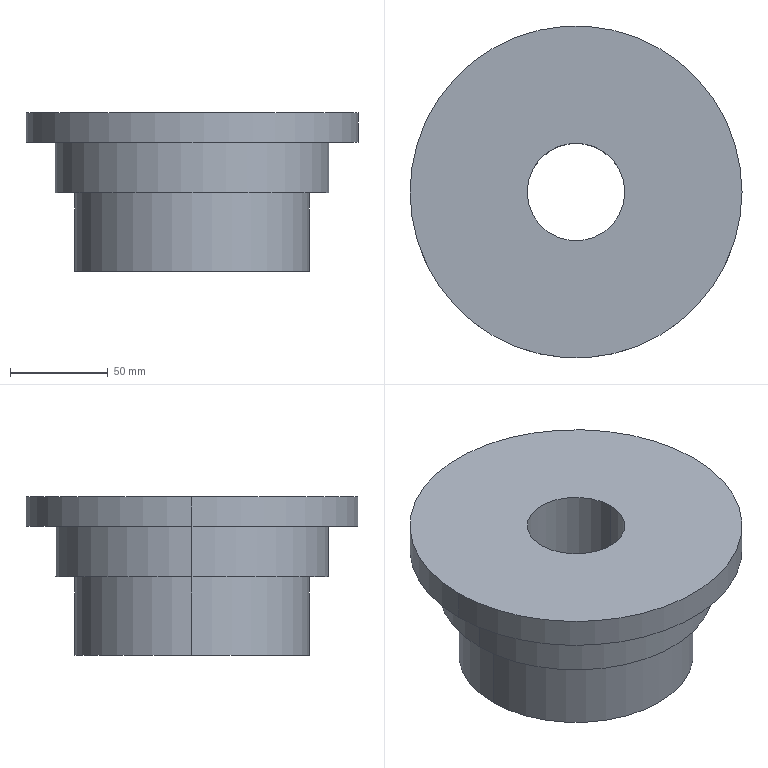Part | SolidWorks | features ICE 2, Cut 1, Extrusion 1 | 1 solid | 12 faces | box 170 x 170 x 81 mm | volume 1034055 mm3 | cylinder 8 | plane 4 | commonest cylinder face diameters 50 x2 120 x2 140 x2 170 x2
STEP:
#1=CARTESIAN_POINT('',(-25.,0.,-40.));
#2=VERTEX_POINT('',#1);
#3=CARTESIAN_POINT('',(25.,0.,-40.));
#4=VERTEX_POINT('',#3);
#5=CARTESIAN_POINT('',(0.,0.,-40.));
#6=DIRECTION('',(0.,0.,1.));
#7=DIRECTION('',(1.,0.,0.));
#8=AXIS2_PLACEMENT_3D('',#5,#6,#7);
#9=CIRCLE('',#8,25.);
#10=EDGE_CURVE('',#2,#4,#9,.T.);
#11=ORIENTED_EDGE('',*,*,#10,.F.);
#12=CARTESIAN_POINT('',(-25.,0.,41.));
#13=VERTEX_POINT('',#12);
#14=CARTESIAN_POINT('',(-25.,0.,-40.));
#15=DIRECTION('',(0.,0.,1.));
#16=VECTOR('',#15,1000.);
#17=LINE('',#14,#16);
#18=EDGE_CURVE('',#2,#13,#17,.T.);
#19=ORIENTED_EDGE('',*,*,#18,.T.);
#20=CARTESIAN_POINT('',(25.,0.,41.));
#21=VERTEX_POINT('',#20);
#22=CARTESIAN_POINT('',(0.,0.,41.));
#23=DIRECTION('',(0.,0.,1.));
#24=DIRECTION('',(1.,0.,0.));
#25=AXIS2_PLACEMENT_3D('',#22,#23,#24);
#26=CIRCLE('',#25,25.);
#27=EDGE_CURVE('',#13,#21,#26,.T.);
#28=ORIENTED_EDGE('',*,*,#27,.T.);
#29=CARTESIAN_POINT('',(25.,0.,-40.));
#30=DIRECTION('',(0.,0.,1.));
#31=VECTOR('',#30,1000.);
#32=LINE('',#29,#31);
#33=EDGE_CURVE('',#4,#21,#32,.T.);
#34=ORIENTED_EDGE('',*,*,#33,.F.);
#35=EDGE_LOOP('',(#11,#19,#28,#34));
#36=FACE_OUTER_BOUND('',#35,.T.);
#37=CARTESIAN_POINT('',(0.,0.,-40.));
#38=DIRECTION('',(0.,0.,1.));
#39=DIRECTION('',(1.,0.,0.));
#40=AXIS2_PLACEMENT_3D('',#37,#38,#39);
#41=CYLINDRICAL_SURFACE('',#40,25.);
#42=ADVANCED_FACE('',(#36),#41,.F.);
#43=CARTESIAN_POINT('',(-60.,0.,-40.));
#44=VERTEX_POINT('',#43);
#45=CARTESIAN_POINT('',(60.,0.,-40.));
#46=VERTEX_POINT('',#45);
#47=CARTESIAN_POINT('',(0.,0.,-40.));
#48=DIRECTION('',(0.,0.,-1.));
#49=DIRECTION('',(-1.,0.,0.));
#50=AXIS2_PLACEMENT_3D('',#47,#48,#49);
#51=CIRCLE('',#50,60.);
#52=EDGE_CURVE('',#44,#46,#51,.T.);
#53=ORIENTED_EDGE('',*,*,#52,.F.);
#54=CARTESIAN_POINT('',(-60.,0.,0.));
#55=VERTEX_POINT('',#54);
#56=CARTESIAN_POINT('',(-60.,0.,-40.));
#57=DIRECTION('',(0.,0.,1.));
#58=VECTOR('',#57,1000.);
#59=LINE('',#56,#58);
#60=EDGE_CURVE('',#44,#55,#59,.T.);
#61=ORIENTED_EDGE('',*,*,#60,.T.);
#62=CARTESIAN_POINT('',(60.,0.,0.));
#63=VERTEX_POINT('',#62);
#64=CARTESIAN_POINT('',(0.,0.,0.));
#65=DIRECTION('',(0.,0.,-1.));
#66=DIRECTION('',(-1.,0.,0.));
#67=AXIS2_PLACEMENT_3D('',#64,#65,#66);
#68=CIRCLE('',#67,60.);
#69=EDGE_CURVE('',#55,#63,#68,.T.);
#70=ORIENTED_EDGE('',*,*,#69,.T.);
#71=CARTESIAN_POINT('',(60.,0.,-40.));
#72=DIRECTION('',(0.,0.,1.));
#73=VECTOR('',#72,1000.);
#74=LINE('',#71,#73);
#75=EDGE_CURVE('',#46,#63,#74,.T.);
#76=ORIENTED_EDGE('',*,*,#75,.F.);
#77=EDGE_LOOP('',(#53,#61,#70,#76));
#78=FACE_OUTER_BOUND('',#77,.T.);
#79=CARTESIAN_POINT('',(0.,0.,-40.));
#80=DIRECTION('',(0.,0.,1.));
#81=DIRECTION('',(1.,0.,0.));
#82=AXIS2_PLACEMENT_3D('',#79,#80,#81);
#83=CYLINDRICAL_SURFACE('',#82,60.);
#84=ADVANCED_FACE('',(#78),#83,.T.);
#85=CARTESIAN_POINT('',(85.,0.,41.));
#86=VERTEX_POINT('',#85);
#87=CARTESIAN_POINT('',(-85.,0.,41.));
#88=VERTEX_POINT('',#87);
#89=CARTESIAN_POINT('',(0.,0.,41.));
#90=DIRECTION('',(0.,0.,1.));
#91=DIRECTION('',(1.,0.,0.));
#92=AXIS2_PLACEMENT_3D('',#89,#90,#91);
#93=CIRCLE('',#92,85.);
#94=EDGE_CURVE('',#86,#88,#93,.T.);
#95=ORIENTED_EDGE('',*,*,#94,.F.);
#96=CARTESIAN_POINT('',(85.,0.,26.));
#97=VERTEX_POINT('',#96);
#98=CARTESIAN_POINT('',(85.,0.,41.));
#99=DIRECTION('',(0.,0.,-1.));
#100=VECTOR('',#99,1000.);
#101=LINE('',#98,#100);
#102=EDGE_CURVE('',#86,#97,#101,.T.);
#103=ORIENTED_EDGE('',*,*,#102,.T.);
#104=CARTESIAN_POINT('',(-85.,0.,26.));
#105=VERTEX_POINT('',#104);
#106=CARTESIAN_POINT('',(0.,0.,26.));
#107=DIRECTION('',(0.,0.,1.));
#108=DIRECTION('',(1.,0.,0.));
#109=AXIS2_PLACEMENT_3D('',#106,#107,#108);
#110=CIRCLE('',#109,85.);
#111=EDGE_CURVE('',#97,#105,#110,.T.);
#112=ORIENTED_EDGE('',*,*,#111,.T.);
#113=CARTESIAN_POINT('',(-85.,0.,41.));
#114=DIRECTION('',(0.,0.,-1.));
#115=VECTOR('',#114,1000.);
#116=LINE('',#113,#115);
#117=EDGE_CURVE('',#88,#105,#116,.T.);
#118=ORIENTED_EDGE('',*,*,#117,.F.);
#119=EDGE_LOOP('',(#95,#103,#112,#118));
#120=FACE_OUTER_BOUND('',#119,.T.);
#121=CARTESIAN_POINT('',(0.,0.,41.));
#122=DIRECTION('',(0.,0.,-1.));
#123=DIRECTION('',(-1.,0.,0.));
#124=AXIS2_PLACEMENT_3D('',#121,#122,#123);
#125=CYLINDRICAL_SURFACE('',#124,85.);
#126=ADVANCED_FACE('',(#120),#125,.T.);
#127=CARTESIAN_POINT('',(70.,0.,26.));
#128=VERTEX_POINT('',#127);
#129=CARTESIAN_POINT('',(-70.,0.,26.));
#130=VERTEX_POINT('',#129);
#131=CARTESIAN_POINT('',(0.,0.,26.));
#132=DIRECTION('',(0.,0.,1.));
#133=DIRECTION('',(1.,0.,0.));
#134=AXIS2_PLACEMENT_3D('',#131,#132,#133);
#135=CIRCLE('',#134,70.);
#136=EDGE_CURVE('',#128,#130,#135,.T.);
#137=ORIENTED_EDGE('',*,*,#136,.F.);
#138=CARTESIAN_POINT('',(70.,0.,0.));
#139=VERTEX_POINT('',#138);
#140=CARTESIAN_POINT('',(70.,0.,223.99));
#141=DIRECTION('',(0.,0.,-1.));
#142=VECTOR('',#141,1000.);
#143=LINE('',#140,#142);
#144=EDGE_CURVE('',#128,#139,#143,.T.);
#145=ORIENTED_EDGE('',*,*,#144,.T.);
#146=CARTESIAN_POINT('',(-70.,0.,0.));
#147=VERTEX_POINT('',#146);
#148=CARTESIAN_POINT('',(0.,0.,0.));
#149=DIRECTION('',(0.,0.,1.));
#150=DIRECTION('',(1.,0.,0.));
#151=AXIS2_PLACEMENT_3D('',#148,#149,#150);
#152=CIRCLE('',#151,70.);
#153=EDGE_CURVE('',#139,#147,#152,.T.);
#154=ORIENTED_EDGE('',*,*,#153,.T.);
#155=CARTESIAN_POINT('',(-70.,0.,223.99));
#156=DIRECTION('',(0.,0.,-1.));
#157=VECTOR('',#156,1000.);
#158=LINE('',#155,#157);
#159=EDGE_CURVE('',#130,#147,#158,.T.);
#160=ORIENTED_EDGE('',*,*,#159,.F.);
#161=EDGE_LOOP('',(#137,#145,#154,#160));
#162=FACE_OUTER_BOUND('',#161,.T.);
#163=CARTESIAN_POINT('',(0.,0.,223.99));
#164=DIRECTION('',(0.,0.,-1.));
#165=DIRECTION('',(-1.,0.,0.));
#166=AXIS2_PLACEMENT_3D('',#163,#164,#165);
#167=CYLINDRICAL_SURFACE('',#166,70.);
#168=ADVANCED_FACE('',(#162),#167,.T.);
#169=ORIENTED_EDGE('',*,*,#144,.F.);
#170=CARTESIAN_POINT('',(0.,0.,26.));
#171=DIRECTION('',(0.,0.,1.));
#172=DIRECTION('',(1.,0.,0.));
#173=AXIS2_PLACEMENT_3D('',#170,#171,#172);
#174=CIRCLE('',#173,70.);
#175=EDGE_CURVE('',#130,#128,#174,.T.);
#176=ORIENTED_EDGE('',*,*,#175,.F.);
#177=ORIENTED_EDGE('',*,*,#159,.T.);
#178=CARTESIAN_POINT('',(0.,0.,0.));
#179=DIRECTION('',(0.,0.,1.));
#180=DIRECTION('',(1.,0.,0.));
#181=AXIS2_PLACEMENT_3D('',#178,#179,#180);
#182=CIRCLE('',#181,70.);
#183=EDGE_CURVE('',#147,#139,#182,.T.);
#184=ORIENTED_EDGE('',*,*,#183,.T.);
#185=EDGE_LOOP('',(#169,#176,#177,#184));
#186=FACE_OUTER_BOUND('',#185,.T.);
#187=CARTESIAN_POINT('',(0.,0.,223.99));
#188=DIRECTION('',(0.,0.,-1.));
#189=DIRECTION('',(-1.,0.,0.));
#190=AXIS2_PLACEMENT_3D('',#187,#188,#189);
#191=CYLINDRICAL_SURFACE('',#190,70.);
#192=ADVANCED_FACE('',(#186),#191,.T.);
#193=CARTESIAN_POINT('',(0.,0.,0.));
#194=DIRECTION('',(0.,0.,-1.));
#195=DIRECTION('',(-1.,0.,0.));
#196=AXIS2_PLACEMENT_3D('',#193,#194,#195);
#197=CIRCLE('',#196,60.);
#198=EDGE_CURVE('',#63,#55,#197,.T.);
#199=ORIENTED_EDGE('',*,*,#198,.F.);
#200=ORIENTED_EDGE('',*,*,#69,.F.);
#201=EDGE_LOOP('',(#199,#200));
#202=FACE_BOUND('',#201,.T.);
#203=ORIENTED_EDGE('',*,*,#183,.F.);
#204=ORIENTED_EDGE('',*,*,#153,.F.);
#205=EDGE_LOOP('',(#203,#204));
#206=FACE_OUTER_BOUND('',#205,.T.);
#207=CARTESIAN_POINT('',(0.,0.,0.));
#208=DIRECTION('',(0.,0.,1.));
#209=DIRECTION('',(1.,0.,0.));
#210=AXIS2_PLACEMENT_3D('',#207,#208,#209);
#211=PLANE('',#210);
#212=ADVANCED_FACE('',(#202,#206),#211,.F.);
#213=ORIENTED_EDGE('',*,*,#102,.F.);
#214=CARTESIAN_POINT('',(0.,0.,41.));
#215=DIRECTION('',(0.,0.,1.));
#216=DIRECTION('',(1.,0.,0.));
#217=AXIS2_PLACEMENT_3D('',#214,#215,#216);
#218=CIRCLE('',#217,85.);
#219=EDGE_CURVE('',#88,#86,#218,.T.);
#220=ORIENTED_EDGE('',*,*,#219,.F.);
#221=ORIENTED_EDGE('',*,*,#117,.T.);
#222=CARTESIAN_POINT('',(0.,0.,26.));
#223=DIRECTION('',(0.,0.,1.));
#224=DIRECTION('',(1.,0.,0.));
#225=AXIS2_PLACEMENT_3D('',#222,#223,#224);
#226=CIRCLE('',#225,85.);
#227=EDGE_CURVE('',#105,#97,#226,.T.);
#228=ORIENTED_EDGE('',*,*,#227,.T.);
#229=EDGE_LOOP('',(#213,#220,#221,#228));
#230=FACE_OUTER_BOUND('',#229,.T.);
#231=CARTESIAN_POINT('',(0.,0.,41.));
#232=DIRECTION('',(0.,0.,-1.));
#233=DIRECTION('',(-1.,0.,0.));
#234=AXIS2_PLACEMENT_3D('',#231,#232,#233);
#235=CYLINDRICAL_SURFACE('',#234,85.);
#236=ADVANCED_FACE('',(#230),#235,.T.);
#237=CARTESIAN_POINT('',(0.,0.,41.));
#238=DIRECTION('',(0.,0.,1.));
#239=DIRECTION('',(1.,0.,0.));
#240=AXIS2_PLACEMENT_3D('',#237,#238,#239);
#241=CIRCLE('',#240,25.);
#242=EDGE_CURVE('',#21,#13,#241,.T.);
#243=ORIENTED_EDGE('',*,*,#242,.F.);
#244=ORIENTED_EDGE('',*,*,#27,.F.);
#245=EDGE_LOOP('',(#243,#244));
#246=FACE_BOUND('',#245,.T.);
#247=ORIENTED_EDGE('',*,*,#219,.T.);
#248=ORIENTED_EDGE('',*,*,#94,.T.);
#249=EDGE_LOOP('',(#247,#248));
#250=FACE_OUTER_BOUND('',#249,.T.);
#251=CARTESIAN_POINT('',(0.,0.,41.));
#252=DIRECTION('',(0.,0.,1.));
#253=DIRECTION('',(1.,0.,0.));
#254=AXIS2_PLACEMENT_3D('',#251,#252,#253);
#255=PLANE('',#254);
#256=ADVANCED_FACE('',(#246,#250),#255,.T.);
#257=ORIENTED_EDGE('',*,*,#175,.T.);
#258=ORIENTED_EDGE('',*,*,#136,.T.);
#259=EDGE_LOOP('',(#257,#258));
#260=FACE_BOUND('',#259,.T.);
#261=ORIENTED_EDGE('',*,*,#227,.F.);
#262=ORIENTED_EDGE('',*,*,#111,.F.);
#263=EDGE_LOOP('',(#261,#262));
#264=FACE_OUTER_BOUND('',#263,.T.);
#265=CARTESIAN_POINT('',(0.,0.,26.));
#266=DIRECTION('',(0.,0.,1.));
#267=DIRECTION('',(1.,0.,0.));
#268=AXIS2_PLACEMENT_3D('',#265,#266,#267);
#269=PLANE('',#268);
#270=ADVANCED_FACE('',(#260,#264),#269,.F.);
#271=ORIENTED_EDGE('',*,*,#60,.F.);
#272=CARTESIAN_POINT('',(0.,0.,-40.));
#273=DIRECTION('',(0.,0.,-1.));
#274=DIRECTION('',(-1.,0.,0.));
#275=AXIS2_PLACEMENT_3D('',#272,#273,#274);
#276=CIRCLE('',#275,60.);
#277=EDGE_CURVE('',#46,#44,#276,.T.);
#278=ORIENTED_EDGE('',*,*,#277,.F.);
#279=ORIENTED_EDGE('',*,*,#75,.T.);
#280=ORIENTED_EDGE('',*,*,#198,.T.);
#281=EDGE_LOOP('',(#271,#278,#279,#280));
#282=FACE_OUTER_BOUND('',#281,.T.);
#283=CARTESIAN_POINT('',(0.,0.,-40.));
#284=DIRECTION('',(0.,0.,1.));
#285=DIRECTION('',(1.,0.,0.));
#286=AXIS2_PLACEMENT_3D('',#283,#284,#285);
#287=CYLINDRICAL_SURFACE('',#286,60.);
#288=ADVANCED_FACE('',(#282),#287,.T.);
#289=CARTESIAN_POINT('',(0.,0.,-40.));
#290=DIRECTION('',(0.,0.,1.));
#291=DIRECTION('',(1.,0.,0.));
#292=AXIS2_PLACEMENT_3D('',#289,#290,#291);
#293=CIRCLE('',#292,25.);
#294=EDGE_CURVE('',#4,#2,#293,.T.);
#295=ORIENTED_EDGE('',*,*,#294,.T.);
#296=ORIENTED_EDGE('',*,*,#10,.T.);
#297=EDGE_LOOP('',(#295,#296));
#298=FACE_BOUND('',#297,.T.);
#299=ORIENTED_EDGE('',*,*,#277,.T.);
#300=ORIENTED_EDGE('',*,*,#52,.T.);
#301=EDGE_LOOP('',(#299,#300));
#302=FACE_OUTER_BOUND('',#301,.T.);
#303=CARTESIAN_POINT('',(0.,0.,-40.));
#304=DIRECTION('',(0.,0.,-1.));
#305=DIRECTION('',(-1.,0.,0.));
#306=AXIS2_PLACEMENT_3D('',#303,#304,#305);
#307=PLANE('',#306);
#308=ADVANCED_FACE('',(#298,#302),#307,.T.);
#309=ORIENTED_EDGE('',*,*,#18,.F.);
#310=ORIENTED_EDGE('',*,*,#294,.F.);
#311=ORIENTED_EDGE('',*,*,#33,.T.);
#312=ORIENTED_EDGE('',*,*,#242,.T.);
#313=EDGE_LOOP('',(#309,#310,#311,#312));
#314=FACE_OUTER_BOUND('',#313,.T.);
#315=CARTESIAN_POINT('',(0.,0.,-40.));
#316=DIRECTION('',(0.,0.,1.));
#317=DIRECTION('',(1.,0.,0.));
#318=AXIS2_PLACEMENT_3D('',#315,#316,#317);
#319=CYLINDRICAL_SURFACE('',#318,25.);
#320=ADVANCED_FACE('',(#314),#319,.F.);
#321=CLOSED_SHELL('',(#42,#84,#126,#168,#192,#212,#236,#256,#270,#288,#308,#320));
#322=MANIFOLD_SOLID_BREP('',#321);
#323=CARTESIAN_POINT('',(0.,0.,0.));
#324=DIRECTION('',(0.,0.,1.));
#325=DIRECTION('',(1.,0.,0.));
#326=AXIS2_PLACEMENT_3D('',#323,#324,#325);
#327=(LENGTH_UNIT()NAMED_UNIT(*)SI_UNIT(.MILLI.,.METRE.));
#328=UNCERTAINTY_MEASURE_WITH_UNIT(LENGTH_MEASURE(0.00001),#327,'','');
#329=(NAMED_UNIT(*)PLANE_ANGLE_UNIT()SI_UNIT($,.RADIAN.));
#330=(NAMED_UNIT(*)SI_UNIT($,.STERADIAN.)SOLID_ANGLE_UNIT());
#331=(GEOMETRIC_REPRESENTATION_CONTEXT(3)GLOBAL_UNCERTAINTY_ASSIGNED_CONTEXT((#328))GLOBAL_UNIT_ASSIGNED_CONTEXT((#327,#329,#330))REPRESENTATION_CONTEXT('',''));
#332=ADVANCED_BREP_SHAPE_REPRESENTATION('',(#322,#326),#331);